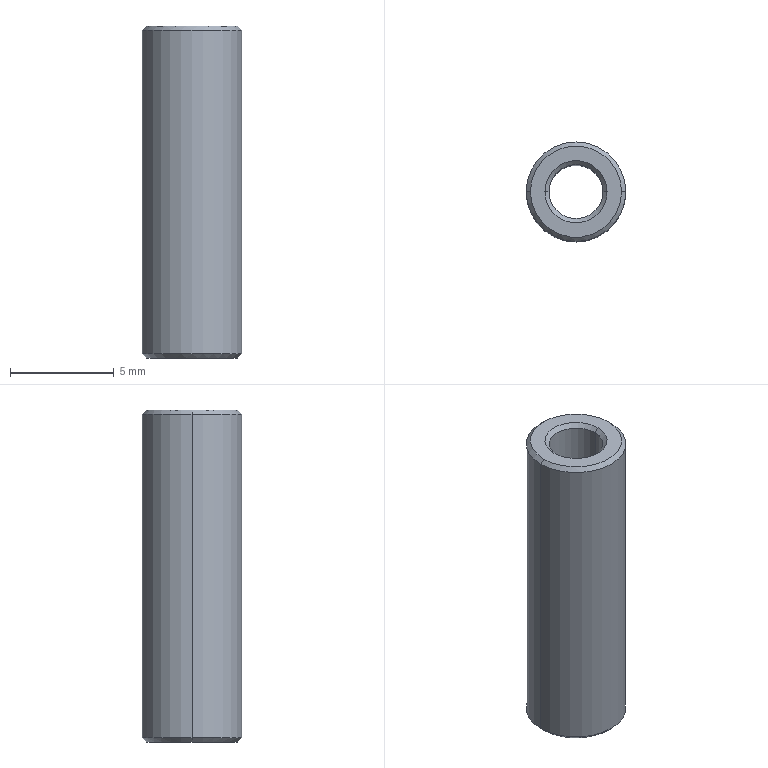Part | SolidWorks | features Revolution 1 | 1 solid | 14 faces | box 4.8 x 4.8 x 16 mm | volume 203.651 mm3 | cone 8 | cylinder 4 | plane 2 | commonest cylinder face diameters 2.6 x2 4.8 x2
STEP:
#1=CARTESIAN_POINT('',(-1.3,0.,-15.8));
#2=VERTEX_POINT('',#1);
#3=CARTESIAN_POINT('',(1.3,0.,-15.8));
#4=VERTEX_POINT('',#3);
#5=CARTESIAN_POINT('',(0.,0.,-15.8));
#6=DIRECTION('',(0.,0.,1.));
#7=DIRECTION('',(1.,0.,0.));
#8=AXIS2_PLACEMENT_3D('',#5,#6,#7);
#9=CIRCLE('',#8,1.3);
#10=EDGE_CURVE('',#2,#4,#9,.T.);
#11=ORIENTED_EDGE('',*,*,#10,.F.);
#12=CARTESIAN_POINT('',(-1.3,0.,-0.2));
#13=VERTEX_POINT('',#12);
#14=CARTESIAN_POINT('',(-1.3,0.,0.));
#15=DIRECTION('',(0.,0.,1.));
#16=VECTOR('',#15,1000.);
#17=LINE('',#14,#16);
#18=EDGE_CURVE('',#2,#13,#17,.T.);
#19=ORIENTED_EDGE('',*,*,#18,.T.);
#20=CARTESIAN_POINT('',(1.3,0.,-0.2));
#21=VERTEX_POINT('',#20);
#22=CARTESIAN_POINT('',(0.,0.,-0.2));
#23=DIRECTION('',(0.,0.,1.));
#24=DIRECTION('',(1.,0.,0.));
#25=AXIS2_PLACEMENT_3D('',#22,#23,#24);
#26=CIRCLE('',#25,1.3);
#27=EDGE_CURVE('',#13,#21,#26,.T.);
#28=ORIENTED_EDGE('',*,*,#27,.T.);
#29=CARTESIAN_POINT('',(1.3,0.,0.));
#30=DIRECTION('',(0.,0.,1.));
#31=VECTOR('',#30,1000.);
#32=LINE('',#29,#31);
#33=EDGE_CURVE('',#4,#21,#32,.T.);
#34=ORIENTED_EDGE('',*,*,#33,.F.);
#35=EDGE_LOOP('',(#11,#19,#28,#34));
#36=FACE_OUTER_BOUND('',#35,.T.);
#37=CARTESIAN_POINT('',(0.,0.,0.));
#38=DIRECTION('',(0.,0.,1.));
#39=DIRECTION('',(1.,0.,0.));
#40=AXIS2_PLACEMENT_3D('',#37,#38,#39);
#41=CYLINDRICAL_SURFACE('',#40,1.3);
#42=ADVANCED_FACE('',(#36),#41,.F.);
#43=ORIENTED_EDGE('',*,*,#10,.T.);
#44=CARTESIAN_POINT('',(1.5,0.,-16.));
#45=VERTEX_POINT('',#44);
#46=CARTESIAN_POINT('',(1.5,0.,-16.));
#47=DIRECTION('',(0.7071,0.,-0.7071));
#48=VECTOR('',#47,1000.);
#49=LINE('',#46,#48);
#50=EDGE_CURVE('',#4,#45,#49,.T.);
#51=ORIENTED_EDGE('',*,*,#50,.T.);
#52=CARTESIAN_POINT('',(-1.5,0.,-16.));
#53=VERTEX_POINT('',#52);
#54=CARTESIAN_POINT('',(0.,0.,-16.));
#55=DIRECTION('',(0.,0.,1.));
#56=DIRECTION('',(1.,0.,0.));
#57=AXIS2_PLACEMENT_3D('',#54,#55,#56);
#58=CIRCLE('',#57,1.5);
#59=EDGE_CURVE('',#53,#45,#58,.T.);
#60=ORIENTED_EDGE('',*,*,#59,.F.);
#61=CARTESIAN_POINT('',(-1.5,0.,-16.));
#62=DIRECTION('',(-0.7071,0.,-0.7071));
#63=VECTOR('',#62,1000.);
#64=LINE('',#61,#63);
#65=EDGE_CURVE('',#2,#53,#64,.T.);
#66=ORIENTED_EDGE('',*,*,#65,.F.);
#67=EDGE_LOOP('',(#43,#51,#60,#66));
#68=FACE_OUTER_BOUND('',#67,.T.);
#69=CARTESIAN_POINT('',(0.,0.,-16.));
#70=DIRECTION('',(0.,0.,-1.));
#71=DIRECTION('',(-1.,0.,0.));
#72=AXIS2_PLACEMENT_3D('',#69,#70,#71);
#73=CONICAL_SURFACE('',#72,1.5,0.7854);
#74=ADVANCED_FACE('',(#68),#73,.F.);
#75=CARTESIAN_POINT('',(2.2,0.,-16.));
#76=VERTEX_POINT('',#75);
#77=CARTESIAN_POINT('',(-2.2,0.,-16.));
#78=VERTEX_POINT('',#77);
#79=CARTESIAN_POINT('',(0.,0.,-16.));
#80=DIRECTION('',(0.,0.,1.));
#81=DIRECTION('',(1.,0.,0.));
#82=AXIS2_PLACEMENT_3D('',#79,#80,#81);
#83=CIRCLE('',#82,2.2);
#84=EDGE_CURVE('',#76,#78,#83,.T.);
#85=ORIENTED_EDGE('',*,*,#84,.T.);
#86=CARTESIAN_POINT('',(-2.4,0.,-15.8));
#87=VERTEX_POINT('',#86);
#88=CARTESIAN_POINT('',(-2.4,0.,-15.8));
#89=DIRECTION('',(-0.7071,0.,0.7071));
#90=VECTOR('',#89,1000.);
#91=LINE('',#88,#90);
#92=EDGE_CURVE('',#78,#87,#91,.T.);
#93=ORIENTED_EDGE('',*,*,#92,.T.);
#94=CARTESIAN_POINT('',(2.4,0.,-15.8));
#95=VERTEX_POINT('',#94);
#96=CARTESIAN_POINT('',(0.,0.,-15.8));
#97=DIRECTION('',(0.,0.,1.));
#98=DIRECTION('',(1.,0.,0.));
#99=AXIS2_PLACEMENT_3D('',#96,#97,#98);
#100=CIRCLE('',#99,2.4);
#101=EDGE_CURVE('',#95,#87,#100,.T.);
#102=ORIENTED_EDGE('',*,*,#101,.F.);
#103=CARTESIAN_POINT('',(2.4,0.,-15.8));
#104=DIRECTION('',(0.7071,0.,0.7071));
#105=VECTOR('',#104,1000.);
#106=LINE('',#103,#105);
#107=EDGE_CURVE('',#76,#95,#106,.T.);
#108=ORIENTED_EDGE('',*,*,#107,.F.);
#109=EDGE_LOOP('',(#85,#93,#102,#108));
#110=FACE_OUTER_BOUND('',#109,.T.);
#111=CARTESIAN_POINT('',(0.,0.,-15.8));
#112=DIRECTION('',(0.,0.,1.));
#113=DIRECTION('',(1.,0.,0.));
#114=AXIS2_PLACEMENT_3D('',#111,#112,#113);
#115=CONICAL_SURFACE('',#114,2.4,0.7854);
#116=ADVANCED_FACE('',(#110),#115,.T.);
#117=ORIENTED_EDGE('',*,*,#101,.T.);
#118=CARTESIAN_POINT('',(-2.4,0.,-0.2));
#119=VERTEX_POINT('',#118);
#120=CARTESIAN_POINT('',(-2.4,0.,0.));
#121=DIRECTION('',(0.,0.,1.));
#122=VECTOR('',#121,1000.);
#123=LINE('',#120,#122);
#124=EDGE_CURVE('',#87,#119,#123,.T.);
#125=ORIENTED_EDGE('',*,*,#124,.T.);
#126=CARTESIAN_POINT('',(2.4,0.,-0.2));
#127=VERTEX_POINT('',#126);
#128=CARTESIAN_POINT('',(0.,0.,-0.2));
#129=DIRECTION('',(0.,0.,1.));
#130=DIRECTION('',(1.,0.,0.));
#131=AXIS2_PLACEMENT_3D('',#128,#129,#130);
#132=CIRCLE('',#131,2.4);
#133=EDGE_CURVE('',#127,#119,#132,.T.);
#134=ORIENTED_EDGE('',*,*,#133,.F.);
#135=CARTESIAN_POINT('',(2.4,0.,0.));
#136=DIRECTION('',(0.,0.,1.));
#137=VECTOR('',#136,1000.);
#138=LINE('',#135,#137);
#139=EDGE_CURVE('',#95,#127,#138,.T.);
#140=ORIENTED_EDGE('',*,*,#139,.F.);
#141=EDGE_LOOP('',(#117,#125,#134,#140));
#142=FACE_OUTER_BOUND('',#141,.T.);
#143=CARTESIAN_POINT('',(0.,0.,0.));
#144=DIRECTION('',(0.,0.,1.));
#145=DIRECTION('',(1.,0.,0.));
#146=AXIS2_PLACEMENT_3D('',#143,#144,#145);
#147=CYLINDRICAL_SURFACE('',#146,2.4);
#148=ADVANCED_FACE('',(#142),#147,.T.);
#149=CARTESIAN_POINT('',(2.2,0.,0.));
#150=VERTEX_POINT('',#149);
#151=CARTESIAN_POINT('',(-2.2,0.,0.));
#152=VERTEX_POINT('',#151);
#153=CARTESIAN_POINT('',(0.,0.,0.));
#154=DIRECTION('',(0.,0.,1.));
#155=DIRECTION('',(1.,0.,0.));
#156=AXIS2_PLACEMENT_3D('',#153,#154,#155);
#157=CIRCLE('',#156,2.2);
#158=EDGE_CURVE('',#150,#152,#157,.T.);
#159=ORIENTED_EDGE('',*,*,#158,.F.);
#160=CARTESIAN_POINT('',(2.2,0.,0.));
#161=DIRECTION('',(0.7071,0.,-0.7071));
#162=VECTOR('',#161,1000.);
#163=LINE('',#160,#162);
#164=EDGE_CURVE('',#150,#127,#163,.T.);
#165=ORIENTED_EDGE('',*,*,#164,.T.);
#166=ORIENTED_EDGE('',*,*,#133,.T.);
#167=CARTESIAN_POINT('',(-2.2,0.,0.));
#168=DIRECTION('',(-0.7071,0.,-0.7071));
#169=VECTOR('',#168,1000.);
#170=LINE('',#167,#169);
#171=EDGE_CURVE('',#152,#119,#170,.T.);
#172=ORIENTED_EDGE('',*,*,#171,.F.);
#173=EDGE_LOOP('',(#159,#165,#166,#172));
#174=FACE_OUTER_BOUND('',#173,.T.);
#175=CARTESIAN_POINT('',(0.,0.,0.));
#176=DIRECTION('',(0.,0.,-1.));
#177=DIRECTION('',(-1.,0.,0.));
#178=AXIS2_PLACEMENT_3D('',#175,#176,#177);
#179=CONICAL_SURFACE('',#178,2.2,0.7854);
#180=ADVANCED_FACE('',(#174),#179,.T.);
#181=ORIENTED_EDGE('',*,*,#27,.F.);
#182=CARTESIAN_POINT('',(-1.5,0.,0.));
#183=VERTEX_POINT('',#182);
#184=CARTESIAN_POINT('',(-1.3,0.,-0.2));
#185=DIRECTION('',(-0.7071,0.,0.7071));
#186=VECTOR('',#185,1000.);
#187=LINE('',#184,#186);
#188=EDGE_CURVE('',#13,#183,#187,.T.);
#189=ORIENTED_EDGE('',*,*,#188,.T.);
#190=CARTESIAN_POINT('',(1.5,0.,0.));
#191=VERTEX_POINT('',#190);
#192=CARTESIAN_POINT('',(0.,0.,0.));
#193=DIRECTION('',(0.,0.,1.));
#194=DIRECTION('',(1.,0.,0.));
#195=AXIS2_PLACEMENT_3D('',#192,#193,#194);
#196=CIRCLE('',#195,1.5);
#197=EDGE_CURVE('',#183,#191,#196,.T.);
#198=ORIENTED_EDGE('',*,*,#197,.T.);
#199=CARTESIAN_POINT('',(1.3,0.,-0.2));
#200=DIRECTION('',(0.7071,0.,0.7071));
#201=VECTOR('',#200,1000.);
#202=LINE('',#199,#201);
#203=EDGE_CURVE('',#21,#191,#202,.T.);
#204=ORIENTED_EDGE('',*,*,#203,.F.);
#205=EDGE_LOOP('',(#181,#189,#198,#204));
#206=FACE_OUTER_BOUND('',#205,.T.);
#207=CARTESIAN_POINT('',(0.,0.,-0.2));
#208=DIRECTION('',(0.,0.,1.));
#209=DIRECTION('',(1.,0.,0.));
#210=AXIS2_PLACEMENT_3D('',#207,#208,#209);
#211=CONICAL_SURFACE('',#210,1.3,0.7854);
#212=ADVANCED_FACE('',(#206),#211,.F.);
#213=ORIENTED_EDGE('',*,*,#188,.F.);
#214=CARTESIAN_POINT('',(0.,0.,-0.2));
#215=DIRECTION('',(0.,0.,1.));
#216=DIRECTION('',(1.,0.,0.));
#217=AXIS2_PLACEMENT_3D('',#214,#215,#216);
#218=CIRCLE('',#217,1.3);
#219=EDGE_CURVE('',#21,#13,#218,.T.);
#220=ORIENTED_EDGE('',*,*,#219,.F.);
#221=ORIENTED_EDGE('',*,*,#203,.T.);
#222=CARTESIAN_POINT('',(0.,0.,0.));
#223=DIRECTION('',(0.,0.,1.));
#224=DIRECTION('',(1.,0.,0.));
#225=AXIS2_PLACEMENT_3D('',#222,#223,#224);
#226=CIRCLE('',#225,1.5);
#227=EDGE_CURVE('',#191,#183,#226,.T.);
#228=ORIENTED_EDGE('',*,*,#227,.T.);
#229=EDGE_LOOP('',(#213,#220,#221,#228));
#230=FACE_OUTER_BOUND('',#229,.T.);
#231=CARTESIAN_POINT('',(0.,0.,-0.2));
#232=DIRECTION('',(0.,0.,1.));
#233=DIRECTION('',(1.,0.,0.));
#234=AXIS2_PLACEMENT_3D('',#231,#232,#233);
#235=CONICAL_SURFACE('',#234,1.3,0.7854);
#236=ADVANCED_FACE('',(#230),#235,.F.);
#237=CARTESIAN_POINT('',(0.,0.,0.));
#238=DIRECTION('',(0.,0.,1.));
#239=DIRECTION('',(1.,0.,0.));
#240=AXIS2_PLACEMENT_3D('',#237,#238,#239);
#241=CIRCLE('',#240,2.2);
#242=EDGE_CURVE('',#152,#150,#241,.T.);
#243=ORIENTED_EDGE('',*,*,#242,.T.);
#244=ORIENTED_EDGE('',*,*,#158,.T.);
#245=EDGE_LOOP('',(#243,#244));
#246=FACE_OUTER_BOUND('',#245,.T.);
#247=ORIENTED_EDGE('',*,*,#227,.F.);
#248=ORIENTED_EDGE('',*,*,#197,.F.);
#249=EDGE_LOOP('',(#247,#248));
#250=FACE_BOUND('',#249,.T.);
#251=CARTESIAN_POINT('',(1.5,0.,0.));
#252=DIRECTION('',(0.,0.,1.));
#253=DIRECTION('',(1.,0.,0.));
#254=AXIS2_PLACEMENT_3D('',#251,#252,#253);
#255=PLANE('',#254);
#256=ADVANCED_FACE('',(#246,#250),#255,.T.);
#257=ORIENTED_EDGE('',*,*,#164,.F.);
#258=ORIENTED_EDGE('',*,*,#242,.F.);
#259=ORIENTED_EDGE('',*,*,#171,.T.);
#260=CARTESIAN_POINT('',(0.,0.,-0.2));
#261=DIRECTION('',(0.,0.,1.));
#262=DIRECTION('',(1.,0.,0.));
#263=AXIS2_PLACEMENT_3D('',#260,#261,#262);
#264=CIRCLE('',#263,2.4);
#265=EDGE_CURVE('',#119,#127,#264,.T.);
#266=ORIENTED_EDGE('',*,*,#265,.T.);
#267=EDGE_LOOP('',(#257,#258,#259,#266));
#268=FACE_OUTER_BOUND('',#267,.T.);
#269=CARTESIAN_POINT('',(0.,0.,0.));
#270=DIRECTION('',(0.,0.,-1.));
#271=DIRECTION('',(-1.,0.,0.));
#272=AXIS2_PLACEMENT_3D('',#269,#270,#271);
#273=CONICAL_SURFACE('',#272,2.2,0.7854);
#274=ADVANCED_FACE('',(#268),#273,.T.);
#275=ORIENTED_EDGE('',*,*,#124,.F.);
#276=CARTESIAN_POINT('',(0.,0.,-15.8));
#277=DIRECTION('',(0.,0.,1.));
#278=DIRECTION('',(1.,0.,0.));
#279=AXIS2_PLACEMENT_3D('',#276,#277,#278);
#280=CIRCLE('',#279,2.4);
#281=EDGE_CURVE('',#87,#95,#280,.T.);
#282=ORIENTED_EDGE('',*,*,#281,.T.);
#283=ORIENTED_EDGE('',*,*,#139,.T.);
#284=ORIENTED_EDGE('',*,*,#265,.F.);
#285=EDGE_LOOP('',(#275,#282,#283,#284));
#286=FACE_OUTER_BOUND('',#285,.T.);
#287=CARTESIAN_POINT('',(0.,0.,0.));
#288=DIRECTION('',(0.,0.,1.));
#289=DIRECTION('',(1.,0.,0.));
#290=AXIS2_PLACEMENT_3D('',#287,#288,#289);
#291=CYLINDRICAL_SURFACE('',#290,2.4);
#292=ADVANCED_FACE('',(#286),#291,.T.);
#293=ORIENTED_EDGE('',*,*,#92,.F.);
#294=CARTESIAN_POINT('',(0.,0.,-16.));
#295=DIRECTION('',(0.,0.,1.));
#296=DIRECTION('',(1.,0.,0.));
#297=AXIS2_PLACEMENT_3D('',#294,#295,#296);
#298=CIRCLE('',#297,2.2);
#299=EDGE_CURVE('',#78,#76,#298,.T.);
#300=ORIENTED_EDGE('',*,*,#299,.T.);
#301=ORIENTED_EDGE('',*,*,#107,.T.);
#302=ORIENTED_EDGE('',*,*,#281,.F.);
#303=EDGE_LOOP('',(#293,#300,#301,#302));
#304=FACE_OUTER_BOUND('',#303,.T.);
#305=CARTESIAN_POINT('',(0.,0.,-15.8));
#306=DIRECTION('',(0.,0.,1.));
#307=DIRECTION('',(1.,0.,0.));
#308=AXIS2_PLACEMENT_3D('',#305,#306,#307);
#309=CONICAL_SURFACE('',#308,2.4,0.7854);
#310=ADVANCED_FACE('',(#304),#309,.T.);
#311=ORIENTED_EDGE('',*,*,#59,.T.);
#312=CARTESIAN_POINT('',(0.,0.,-16.));
#313=DIRECTION('',(0.,0.,1.));
#314=DIRECTION('',(1.,0.,0.));
#315=AXIS2_PLACEMENT_3D('',#312,#313,#314);
#316=CIRCLE('',#315,1.5);
#317=EDGE_CURVE('',#45,#53,#316,.T.);
#318=ORIENTED_EDGE('',*,*,#317,.T.);
#319=EDGE_LOOP('',(#311,#318));
#320=FACE_BOUND('',#319,.T.);
#321=ORIENTED_EDGE('',*,*,#84,.F.);
#322=ORIENTED_EDGE('',*,*,#299,.F.);
#323=EDGE_LOOP('',(#321,#322));
#324=FACE_OUTER_BOUND('',#323,.T.);
#325=CARTESIAN_POINT('',(1.5,0.,-16.));
#326=DIRECTION('',(0.,0.,-1.));
#327=DIRECTION('',(-1.,0.,0.));
#328=AXIS2_PLACEMENT_3D('',#325,#326,#327);
#329=PLANE('',#328);
#330=ADVANCED_FACE('',(#320,#324),#329,.T.);
#331=ORIENTED_EDGE('',*,*,#50,.F.);
#332=CARTESIAN_POINT('',(0.,0.,-15.8));
#333=DIRECTION('',(0.,0.,1.));
#334=DIRECTION('',(1.,0.,0.));
#335=AXIS2_PLACEMENT_3D('',#332,#333,#334);
#336=CIRCLE('',#335,1.3);
#337=EDGE_CURVE('',#4,#2,#336,.T.);
#338=ORIENTED_EDGE('',*,*,#337,.T.);
#339=ORIENTED_EDGE('',*,*,#65,.T.);
#340=ORIENTED_EDGE('',*,*,#317,.F.);
#341=EDGE_LOOP('',(#331,#338,#339,#340));
#342=FACE_OUTER_BOUND('',#341,.T.);
#343=CARTESIAN_POINT('',(0.,0.,-16.));
#344=DIRECTION('',(0.,0.,-1.));
#345=DIRECTION('',(-1.,0.,0.));
#346=AXIS2_PLACEMENT_3D('',#343,#344,#345);
#347=CONICAL_SURFACE('',#346,1.5,0.7854);
#348=ADVANCED_FACE('',(#342),#347,.F.);
#349=ORIENTED_EDGE('',*,*,#18,.F.);
#350=ORIENTED_EDGE('',*,*,#337,.F.);
#351=ORIENTED_EDGE('',*,*,#33,.T.);
#352=ORIENTED_EDGE('',*,*,#219,.T.);
#353=EDGE_LOOP('',(#349,#350,#351,#352));
#354=FACE_OUTER_BOUND('',#353,.T.);
#355=CARTESIAN_POINT('',(0.,0.,0.));
#356=DIRECTION('',(0.,0.,1.));
#357=DIRECTION('',(1.,0.,0.));
#358=AXIS2_PLACEMENT_3D('',#355,#356,#357);
#359=CYLINDRICAL_SURFACE('',#358,1.3);
#360=ADVANCED_FACE('',(#354),#359,.F.);
#361=CLOSED_SHELL('',(#42,#74,#116,#148,#180,#212,#236,#256,#274,#292,#310,#330,#348,#360));
#362=MANIFOLD_SOLID_BREP('',#361);
#363=CARTESIAN_POINT('',(0.,0.,0.));
#364=DIRECTION('',(0.,0.,1.));
#365=DIRECTION('',(1.,0.,0.));
#366=AXIS2_PLACEMENT_3D('',#363,#364,#365);
#367=(LENGTH_UNIT()NAMED_UNIT(*)SI_UNIT(.MILLI.,.METRE.));
#368=UNCERTAINTY_MEASURE_WITH_UNIT(LENGTH_MEASURE(0.00001),#367,'','');
#369=(NAMED_UNIT(*)PLANE_ANGLE_UNIT()SI_UNIT($,.RADIAN.));
#370=(NAMED_UNIT(*)SI_UNIT($,.STERADIAN.)SOLID_ANGLE_UNIT());
#371=(GEOMETRIC_REPRESENTATION_CONTEXT(3)GLOBAL_UNCERTAINTY_ASSIGNED_CONTEXT((#368))GLOBAL_UNIT_ASSIGNED_CONTEXT((#367,#369,#370))REPRESENTATION_CONTEXT('',''));
#372=ADVANCED_BREP_SHAPE_REPRESENTATION('',(#362,#366),#371);